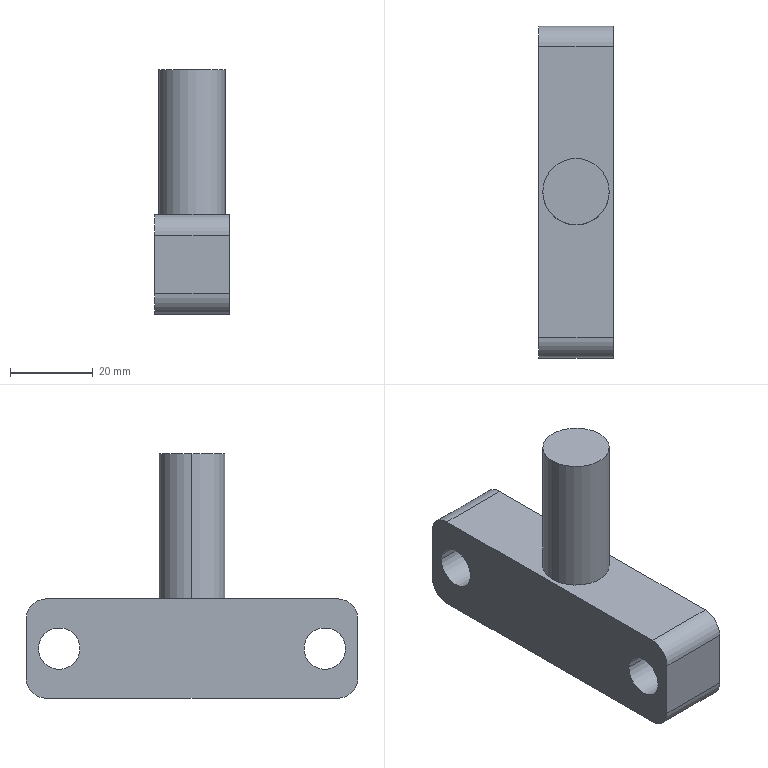Part | SolidWorks | features ICE 2, Extrusion 1, Fillet 1 | 1 solid | 17 faces | box 18 x 80 x 59 mm | volume 38383 mm3 | cylinder 10 | plane 7 | commonest cylinder face diameters 10 x8 16 x2
STEP:
#1=CARTESIAN_POINT('',(9.,37.,-12.));
#2=VERTEX_POINT('',#1);
#3=CARTESIAN_POINT('',(9.,27.,-12.));
#4=VERTEX_POINT('',#3);
#5=CARTESIAN_POINT('',(9.,32.,-12.));
#6=DIRECTION('',(-1.,0.,0.));
#7=DIRECTION('',(0.,-1.,0.));
#8=AXIS2_PLACEMENT_3D('',#5,#6,#7);
#9=CIRCLE('',#8,5.);
#10=EDGE_CURVE('',#2,#4,#9,.T.);
#11=ORIENTED_EDGE('',*,*,#10,.F.);
#12=CARTESIAN_POINT('',(-9.,37.,-12.));
#13=VERTEX_POINT('',#12);
#14=CARTESIAN_POINT('',(9.,37.,-12.));
#15=DIRECTION('',(-1.,0.,0.));
#16=VECTOR('',#15,1000.);
#17=LINE('',#14,#16);
#18=EDGE_CURVE('',#2,#13,#17,.T.);
#19=ORIENTED_EDGE('',*,*,#18,.T.);
#20=CARTESIAN_POINT('',(-9.,27.,-12.));
#21=VERTEX_POINT('',#20);
#22=CARTESIAN_POINT('',(-9.,32.,-12.));
#23=DIRECTION('',(-1.,0.,0.));
#24=DIRECTION('',(0.,-1.,0.));
#25=AXIS2_PLACEMENT_3D('',#22,#23,#24);
#26=CIRCLE('',#25,5.);
#27=EDGE_CURVE('',#13,#21,#26,.T.);
#28=ORIENTED_EDGE('',*,*,#27,.T.);
#29=CARTESIAN_POINT('',(9.,27.,-12.));
#30=DIRECTION('',(-1.,0.,0.));
#31=VECTOR('',#30,1000.);
#32=LINE('',#29,#31);
#33=EDGE_CURVE('',#4,#21,#32,.T.);
#34=ORIENTED_EDGE('',*,*,#33,.F.);
#35=EDGE_LOOP('',(#11,#19,#28,#34));
#36=FACE_OUTER_BOUND('',#35,.T.);
#37=CARTESIAN_POINT('',(9.,32.,-12.));
#38=DIRECTION('',(-1.,0.,0.));
#39=DIRECTION('',(0.,-1.,0.));
#40=AXIS2_PLACEMENT_3D('',#37,#38,#39);
#41=CYLINDRICAL_SURFACE('',#40,5.);
#42=ADVANCED_FACE('',(#36),#41,.F.);
#43=CARTESIAN_POINT('',(9.,-27.,-12.));
#44=VERTEX_POINT('',#43);
#45=CARTESIAN_POINT('',(9.,-37.,-12.));
#46=VERTEX_POINT('',#45);
#47=CARTESIAN_POINT('',(9.,-32.,-12.));
#48=DIRECTION('',(-1.,0.,0.));
#49=DIRECTION('',(0.,-1.,0.));
#50=AXIS2_PLACEMENT_3D('',#47,#48,#49);
#51=CIRCLE('',#50,5.);
#52=EDGE_CURVE('',#44,#46,#51,.T.);
#53=ORIENTED_EDGE('',*,*,#52,.F.);
#54=CARTESIAN_POINT('',(-9.,-27.,-12.));
#55=VERTEX_POINT('',#54);
#56=CARTESIAN_POINT('',(9.,-27.,-12.));
#57=DIRECTION('',(-1.,0.,0.));
#58=VECTOR('',#57,1000.);
#59=LINE('',#56,#58);
#60=EDGE_CURVE('',#44,#55,#59,.T.);
#61=ORIENTED_EDGE('',*,*,#60,.T.);
#62=CARTESIAN_POINT('',(-9.,-37.,-12.));
#63=VERTEX_POINT('',#62);
#64=CARTESIAN_POINT('',(-9.,-32.,-12.));
#65=DIRECTION('',(-1.,0.,0.));
#66=DIRECTION('',(0.,-1.,0.));
#67=AXIS2_PLACEMENT_3D('',#64,#65,#66);
#68=CIRCLE('',#67,5.);
#69=EDGE_CURVE('',#55,#63,#68,.T.);
#70=ORIENTED_EDGE('',*,*,#69,.T.);
#71=CARTESIAN_POINT('',(9.,-37.,-12.));
#72=DIRECTION('',(-1.,0.,0.));
#73=VECTOR('',#72,1000.);
#74=LINE('',#71,#73);
#75=EDGE_CURVE('',#46,#63,#74,.T.);
#76=ORIENTED_EDGE('',*,*,#75,.F.);
#77=EDGE_LOOP('',(#53,#61,#70,#76));
#78=FACE_OUTER_BOUND('',#77,.T.);
#79=CARTESIAN_POINT('',(9.,-32.,-12.));
#80=DIRECTION('',(-1.,0.,0.));
#81=DIRECTION('',(0.,-1.,0.));
#82=AXIS2_PLACEMENT_3D('',#79,#80,#81);
#83=CYLINDRICAL_SURFACE('',#82,5.);
#84=ADVANCED_FACE('',(#78),#83,.F.);
#85=CARTESIAN_POINT('',(8.,0.,35.));
#86=VERTEX_POINT('',#85);
#87=CARTESIAN_POINT('',(-8.,0.,35.));
#88=VERTEX_POINT('',#87);
#89=CARTESIAN_POINT('',(0.,0.,35.));
#90=DIRECTION('',(0.,0.,1.));
#91=DIRECTION('',(1.,0.,0.));
#92=AXIS2_PLACEMENT_3D('',#89,#90,#91);
#93=CIRCLE('',#92,8.);
#94=EDGE_CURVE('',#86,#88,#93,.T.);
#95=ORIENTED_EDGE('',*,*,#94,.F.);
#96=CARTESIAN_POINT('',(8.,0.,0.));
#97=VERTEX_POINT('',#96);
#98=CARTESIAN_POINT('',(8.,0.,35.));
#99=DIRECTION('',(0.,0.,-1.));
#100=VECTOR('',#99,1000.);
#101=LINE('',#98,#100);
#102=EDGE_CURVE('',#86,#97,#101,.T.);
#103=ORIENTED_EDGE('',*,*,#102,.T.);
#104=CARTESIAN_POINT('',(-8.,0.,0.));
#105=VERTEX_POINT('',#104);
#106=CARTESIAN_POINT('',(0.,0.,0.));
#107=DIRECTION('',(0.,0.,1.));
#108=DIRECTION('',(1.,0.,0.));
#109=AXIS2_PLACEMENT_3D('',#106,#107,#108);
#110=CIRCLE('',#109,8.);
#111=EDGE_CURVE('',#97,#105,#110,.T.);
#112=ORIENTED_EDGE('',*,*,#111,.T.);
#113=CARTESIAN_POINT('',(-8.,0.,35.));
#114=DIRECTION('',(0.,0.,-1.));
#115=VECTOR('',#114,1000.);
#116=LINE('',#113,#115);
#117=EDGE_CURVE('',#88,#105,#116,.T.);
#118=ORIENTED_EDGE('',*,*,#117,.F.);
#119=EDGE_LOOP('',(#95,#103,#112,#118));
#120=FACE_OUTER_BOUND('',#119,.T.);
#121=CARTESIAN_POINT('',(0.,0.,35.));
#122=DIRECTION('',(0.,0.,-1.));
#123=DIRECTION('',(-1.,0.,0.));
#124=AXIS2_PLACEMENT_3D('',#121,#122,#123);
#125=CYLINDRICAL_SURFACE('',#124,8.);
#126=ADVANCED_FACE('',(#120),#125,.T.);
#127=ORIENTED_EDGE('',*,*,#102,.F.);
#128=CARTESIAN_POINT('',(0.,0.,35.));
#129=DIRECTION('',(0.,0.,1.));
#130=DIRECTION('',(1.,0.,0.));
#131=AXIS2_PLACEMENT_3D('',#128,#129,#130);
#132=CIRCLE('',#131,8.);
#133=EDGE_CURVE('',#88,#86,#132,.T.);
#134=ORIENTED_EDGE('',*,*,#133,.F.);
#135=ORIENTED_EDGE('',*,*,#117,.T.);
#136=CARTESIAN_POINT('',(0.,0.,0.));
#137=DIRECTION('',(0.,0.,1.));
#138=DIRECTION('',(1.,0.,0.));
#139=AXIS2_PLACEMENT_3D('',#136,#137,#138);
#140=CIRCLE('',#139,8.);
#141=EDGE_CURVE('',#105,#97,#140,.T.);
#142=ORIENTED_EDGE('',*,*,#141,.T.);
#143=EDGE_LOOP('',(#127,#134,#135,#142));
#144=FACE_OUTER_BOUND('',#143,.T.);
#145=CARTESIAN_POINT('',(0.,0.,35.));
#146=DIRECTION('',(0.,0.,-1.));
#147=DIRECTION('',(-1.,0.,0.));
#148=AXIS2_PLACEMENT_3D('',#145,#146,#147);
#149=CYLINDRICAL_SURFACE('',#148,8.);
#150=ADVANCED_FACE('',(#144),#149,.T.);
#151=ORIENTED_EDGE('',*,*,#133,.T.);
#152=ORIENTED_EDGE('',*,*,#94,.T.);
#153=EDGE_LOOP('',(#151,#152));
#154=FACE_OUTER_BOUND('',#153,.T.);
#155=CARTESIAN_POINT('',(0.,0.,35.));
#156=DIRECTION('',(0.,0.,1.));
#157=DIRECTION('',(1.,0.,0.));
#158=AXIS2_PLACEMENT_3D('',#155,#156,#157);
#159=PLANE('',#158);
#160=ADVANCED_FACE('',(#154),#159,.T.);
#161=CARTESIAN_POINT('',(-9.,-35.,0.));
#162=VERTEX_POINT('',#161);
#163=CARTESIAN_POINT('',(-9.,35.,0.));
#164=VERTEX_POINT('',#163);
#165=CARTESIAN_POINT('',(-9.,40.,0.));
#166=DIRECTION('',(0.,1.,0.));
#167=VECTOR('',#166,1000.);
#168=LINE('',#165,#167);
#169=EDGE_CURVE('',#162,#164,#168,.T.);
#170=ORIENTED_EDGE('',*,*,#169,.F.);
#171=CARTESIAN_POINT('',(9.,-35.,0.));
#172=VERTEX_POINT('',#171);
#173=CARTESIAN_POINT('',(9.,-35.,0.));
#174=DIRECTION('',(1.,0.,0.));
#175=VECTOR('',#174,1000.);
#176=LINE('',#173,#175);
#177=EDGE_CURVE('',#162,#172,#176,.T.);
#178=ORIENTED_EDGE('',*,*,#177,.T.);
#179=CARTESIAN_POINT('',(9.,35.,0.));
#180=VERTEX_POINT('',#179);
#181=CARTESIAN_POINT('',(9.,40.,0.));
#182=DIRECTION('',(0.,-1.,0.));
#183=VECTOR('',#182,1000.);
#184=LINE('',#181,#183);
#185=EDGE_CURVE('',#180,#172,#184,.T.);
#186=ORIENTED_EDGE('',*,*,#185,.F.);
#187=CARTESIAN_POINT('',(-9.,35.,0.));
#188=DIRECTION('',(-1.,0.,0.));
#189=VECTOR('',#188,1000.);
#190=LINE('',#187,#189);
#191=EDGE_CURVE('',#180,#164,#190,.T.);
#192=ORIENTED_EDGE('',*,*,#191,.T.);
#193=EDGE_LOOP('',(#170,#178,#186,#192));
#194=FACE_OUTER_BOUND('',#193,.T.);
#195=ORIENTED_EDGE('',*,*,#141,.F.);
#196=ORIENTED_EDGE('',*,*,#111,.F.);
#197=EDGE_LOOP('',(#195,#196));
#198=FACE_BOUND('',#197,.T.);
#199=CARTESIAN_POINT('',(0.,0.,0.));
#200=DIRECTION('',(0.,0.,1.));
#201=DIRECTION('',(1.,0.,0.));
#202=AXIS2_PLACEMENT_3D('',#199,#200,#201);
#203=PLANE('',#202);
#204=ADVANCED_FACE('',(#194,#198),#203,.T.);
#205=CARTESIAN_POINT('',(9.,32.,-12.));
#206=DIRECTION('',(-1.,0.,0.));
#207=DIRECTION('',(0.,-1.,0.));
#208=AXIS2_PLACEMENT_3D('',#205,#206,#207);
#209=CIRCLE('',#208,5.);
#210=EDGE_CURVE('',#4,#2,#209,.T.);
#211=ORIENTED_EDGE('',*,*,#210,.T.);
#212=ORIENTED_EDGE('',*,*,#10,.T.);
#213=EDGE_LOOP('',(#211,#212));
#214=FACE_BOUND('',#213,.T.);
#215=CARTESIAN_POINT('',(9.,-32.,-12.));
#216=DIRECTION('',(-1.,0.,0.));
#217=DIRECTION('',(0.,-1.,0.));
#218=AXIS2_PLACEMENT_3D('',#215,#216,#217);
#219=CIRCLE('',#218,5.);
#220=EDGE_CURVE('',#46,#44,#219,.T.);
#221=ORIENTED_EDGE('',*,*,#220,.T.);
#222=ORIENTED_EDGE('',*,*,#52,.T.);
#223=EDGE_LOOP('',(#221,#222));
#224=FACE_BOUND('',#223,.T.);
#225=ORIENTED_EDGE('',*,*,#185,.T.);
#226=CARTESIAN_POINT('',(9.,-40.,-5.));
#227=VERTEX_POINT('',#226);
#228=CARTESIAN_POINT('',(9.,-35.,-5.));
#229=DIRECTION('',(1.,0.,0.));
#230=DIRECTION('',(0.,-1.,0.));
#231=AXIS2_PLACEMENT_3D('',#228,#229,#230);
#232=CIRCLE('',#231,5.);
#233=EDGE_CURVE('',#172,#227,#232,.T.);
#234=ORIENTED_EDGE('',*,*,#233,.T.);
#235=CARTESIAN_POINT('',(9.,-40.,-19.));
#236=VERTEX_POINT('',#235);
#237=CARTESIAN_POINT('',(9.,-40.,-24.));
#238=DIRECTION('',(0.,0.,1.));
#239=VECTOR('',#238,1000.);
#240=LINE('',#237,#239);
#241=EDGE_CURVE('',#236,#227,#240,.T.);
#242=ORIENTED_EDGE('',*,*,#241,.F.);
#243=CARTESIAN_POINT('',(9.,-35.,-24.));
#244=VERTEX_POINT('',#243);
#245=CARTESIAN_POINT('',(9.,-35.,-19.));
#246=DIRECTION('',(1.,0.,0.));
#247=DIRECTION('',(0.,-1.,0.));
#248=AXIS2_PLACEMENT_3D('',#245,#246,#247);
#249=CIRCLE('',#248,5.);
#250=EDGE_CURVE('',#236,#244,#249,.T.);
#251=ORIENTED_EDGE('',*,*,#250,.T.);
#252=CARTESIAN_POINT('',(9.,35.,-24.));
#253=VERTEX_POINT('',#252);
#254=CARTESIAN_POINT('',(9.,40.,-24.));
#255=DIRECTION('',(0.,-1.,0.));
#256=VECTOR('',#255,1000.);
#257=LINE('',#254,#256);
#258=EDGE_CURVE('',#253,#244,#257,.T.);
#259=ORIENTED_EDGE('',*,*,#258,.F.);
#260=CARTESIAN_POINT('',(9.,40.,-19.));
#261=VERTEX_POINT('',#260);
#262=CARTESIAN_POINT('',(9.,35.,-19.));
#263=DIRECTION('',(1.,0.,0.));
#264=DIRECTION('',(0.,-1.,0.));
#265=AXIS2_PLACEMENT_3D('',#262,#263,#264);
#266=CIRCLE('',#265,5.);
#267=EDGE_CURVE('',#253,#261,#266,.T.);
#268=ORIENTED_EDGE('',*,*,#267,.T.);
#269=CARTESIAN_POINT('',(9.,40.,-5.));
#270=VERTEX_POINT('',#269);
#271=CARTESIAN_POINT('',(9.,40.,-24.));
#272=DIRECTION('',(0.,0.,1.));
#273=VECTOR('',#272,1000.);
#274=LINE('',#271,#273);
#275=EDGE_CURVE('',#261,#270,#274,.T.);
#276=ORIENTED_EDGE('',*,*,#275,.T.);
#277=CARTESIAN_POINT('',(9.,35.,-5.));
#278=DIRECTION('',(1.,0.,0.));
#279=DIRECTION('',(0.,-1.,0.));
#280=AXIS2_PLACEMENT_3D('',#277,#278,#279);
#281=CIRCLE('',#280,5.);
#282=EDGE_CURVE('',#270,#180,#281,.T.);
#283=ORIENTED_EDGE('',*,*,#282,.T.);
#284=EDGE_LOOP('',(#225,#234,#242,#251,#259,#268,#276,#283));
#285=FACE_OUTER_BOUND('',#284,.T.);
#286=CARTESIAN_POINT('',(9.,40.,-24.));
#287=DIRECTION('',(-1.,0.,0.));
#288=DIRECTION('',(0.,-1.,0.));
#289=AXIS2_PLACEMENT_3D('',#286,#287,#288);
#290=PLANE('',#289);
#291=ADVANCED_FACE('',(#214,#224,#285),#290,.F.);
#292=ORIENTED_EDGE('',*,*,#241,.T.);
#293=CARTESIAN_POINT('',(-9.,-40.,-5.));
#294=VERTEX_POINT('',#293);
#295=CARTESIAN_POINT('',(-9.,-40.,-5.));
#296=DIRECTION('',(-1.,0.,0.));
#297=VECTOR('',#296,1000.);
#298=LINE('',#295,#297);
#299=EDGE_CURVE('',#227,#294,#298,.T.);
#300=ORIENTED_EDGE('',*,*,#299,.T.);
#301=CARTESIAN_POINT('',(-9.,-40.,-19.));
#302=VERTEX_POINT('',#301);
#303=CARTESIAN_POINT('',(-9.,-40.,-24.));
#304=DIRECTION('',(0.,0.,1.));
#305=VECTOR('',#304,1000.);
#306=LINE('',#303,#305);
#307=EDGE_CURVE('',#302,#294,#306,.T.);
#308=ORIENTED_EDGE('',*,*,#307,.F.);
#309=CARTESIAN_POINT('',(-9.,-40.,-19.));
#310=DIRECTION('',(1.,0.,0.));
#311=VECTOR('',#310,1000.);
#312=LINE('',#309,#311);
#313=EDGE_CURVE('',#302,#236,#312,.T.);
#314=ORIENTED_EDGE('',*,*,#313,.T.);
#315=EDGE_LOOP('',(#292,#300,#308,#314));
#316=FACE_OUTER_BOUND('',#315,.T.);
#317=CARTESIAN_POINT('',(-9.,-40.,-24.));
#318=DIRECTION('',(0.,1.,0.));
#319=DIRECTION('',(0.,0.,1.));
#320=AXIS2_PLACEMENT_3D('',#317,#318,#319);
#321=PLANE('',#320);
#322=ADVANCED_FACE('',(#316),#321,.F.);
#323=CARTESIAN_POINT('',(-9.,32.,-12.));
#324=DIRECTION('',(-1.,0.,0.));
#325=DIRECTION('',(0.,-1.,0.));
#326=AXIS2_PLACEMENT_3D('',#323,#324,#325);
#327=CIRCLE('',#326,5.);
#328=EDGE_CURVE('',#21,#13,#327,.T.);
#329=ORIENTED_EDGE('',*,*,#328,.F.);
#330=ORIENTED_EDGE('',*,*,#27,.F.);
#331=EDGE_LOOP('',(#329,#330));
#332=FACE_BOUND('',#331,.T.);
#333=CARTESIAN_POINT('',(-9.,-32.,-12.));
#334=DIRECTION('',(-1.,0.,0.));
#335=DIRECTION('',(0.,-1.,0.));
#336=AXIS2_PLACEMENT_3D('',#333,#334,#335);
#337=CIRCLE('',#336,5.);
#338=EDGE_CURVE('',#63,#55,#337,.T.);
#339=ORIENTED_EDGE('',*,*,#338,.F.);
#340=ORIENTED_EDGE('',*,*,#69,.F.);
#341=EDGE_LOOP('',(#339,#340));
#342=FACE_BOUND('',#341,.T.);
#343=ORIENTED_EDGE('',*,*,#307,.T.);
#344=CARTESIAN_POINT('',(-9.,-35.,-5.));
#345=DIRECTION('',(-1.,0.,0.));
#346=DIRECTION('',(0.,1.,0.));
#347=AXIS2_PLACEMENT_3D('',#344,#345,#346);
#348=CIRCLE('',#347,5.);
#349=EDGE_CURVE('',#294,#162,#348,.T.);
#350=ORIENTED_EDGE('',*,*,#349,.T.);
#351=ORIENTED_EDGE('',*,*,#169,.T.);
#352=CARTESIAN_POINT('',(-9.,40.,-5.));
#353=VERTEX_POINT('',#352);
#354=CARTESIAN_POINT('',(-9.,35.,-5.));
#355=DIRECTION('',(-1.,0.,0.));
#356=DIRECTION('',(0.,1.,0.));
#357=AXIS2_PLACEMENT_3D('',#354,#355,#356);
#358=CIRCLE('',#357,5.);
#359=EDGE_CURVE('',#164,#353,#358,.T.);
#360=ORIENTED_EDGE('',*,*,#359,.T.);
#361=CARTESIAN_POINT('',(-9.,40.,-19.));
#362=VERTEX_POINT('',#361);
#363=CARTESIAN_POINT('',(-9.,40.,-24.));
#364=DIRECTION('',(0.,0.,1.));
#365=VECTOR('',#364,1000.);
#366=LINE('',#363,#365);
#367=EDGE_CURVE('',#362,#353,#366,.T.);
#368=ORIENTED_EDGE('',*,*,#367,.F.);
#369=CARTESIAN_POINT('',(-9.,35.,-24.));
#370=VERTEX_POINT('',#369);
#371=CARTESIAN_POINT('',(-9.,35.,-19.));
#372=DIRECTION('',(-1.,0.,0.));
#373=DIRECTION('',(0.,1.,0.));
#374=AXIS2_PLACEMENT_3D('',#371,#372,#373);
#375=CIRCLE('',#374,5.);
#376=EDGE_CURVE('',#362,#370,#375,.T.);
#377=ORIENTED_EDGE('',*,*,#376,.T.);
#378=CARTESIAN_POINT('',(-9.,-35.,-24.));
#379=VERTEX_POINT('',#378);
#380=CARTESIAN_POINT('',(-9.,40.,-24.));
#381=DIRECTION('',(0.,1.,0.));
#382=VECTOR('',#381,1000.);
#383=LINE('',#380,#382);
#384=EDGE_CURVE('',#379,#370,#383,.T.);
#385=ORIENTED_EDGE('',*,*,#384,.F.);
#386=CARTESIAN_POINT('',(-9.,-35.,-19.));
#387=DIRECTION('',(-1.,0.,0.));
#388=DIRECTION('',(0.,1.,0.));
#389=AXIS2_PLACEMENT_3D('',#386,#387,#388);
#390=CIRCLE('',#389,5.);
#391=EDGE_CURVE('',#379,#302,#390,.T.);
#392=ORIENTED_EDGE('',*,*,#391,.T.);
#393=EDGE_LOOP('',(#343,#350,#351,#360,#368,#377,#385,#392));
#394=FACE_OUTER_BOUND('',#393,.T.);
#395=CARTESIAN_POINT('',(-9.,40.,-24.));
#396=DIRECTION('',(1.,0.,0.));
#397=DIRECTION('',(0.,1.,0.));
#398=AXIS2_PLACEMENT_3D('',#395,#396,#397);
#399=PLANE('',#398);
#400=ADVANCED_FACE('',(#332,#342,#394),#399,.F.);
#401=ORIENTED_EDGE('',*,*,#367,.T.);
#402=CARTESIAN_POINT('',(9.,40.,-5.));
#403=DIRECTION('',(1.,0.,0.));
#404=VECTOR('',#403,1000.);
#405=LINE('',#402,#404);
#406=EDGE_CURVE('',#353,#270,#405,.T.);
#407=ORIENTED_EDGE('',*,*,#406,.T.);
#408=ORIENTED_EDGE('',*,*,#275,.F.);
#409=CARTESIAN_POINT('',(-9.,40.,-19.));
#410=DIRECTION('',(-1.,0.,0.));
#411=VECTOR('',#410,1000.);
#412=LINE('',#409,#411);
#413=EDGE_CURVE('',#261,#362,#412,.T.);
#414=ORIENTED_EDGE('',*,*,#413,.T.);
#415=EDGE_LOOP('',(#401,#407,#408,#414));
#416=FACE_OUTER_BOUND('',#415,.T.);
#417=CARTESIAN_POINT('',(-9.,40.,-24.));
#418=DIRECTION('',(0.,-1.,0.));
#419=DIRECTION('',(0.,0.,-1.));
#420=AXIS2_PLACEMENT_3D('',#417,#418,#419);
#421=PLANE('',#420);
#422=ADVANCED_FACE('',(#416),#421,.F.);
#423=ORIENTED_EDGE('',*,*,#258,.T.);
#424=CARTESIAN_POINT('',(0.,-35.,-24.));
#425=DIRECTION('',(-1.,0.,0.));
#426=VECTOR('',#425,1000.);
#427=LINE('',#424,#426);
#428=EDGE_CURVE('',#244,#379,#427,.T.);
#429=ORIENTED_EDGE('',*,*,#428,.T.);
#430=ORIENTED_EDGE('',*,*,#384,.T.);
#431=CARTESIAN_POINT('',(0.,35.,-24.));
#432=DIRECTION('',(1.,0.,0.));
#433=VECTOR('',#432,1000.);
#434=LINE('',#431,#433);
#435=EDGE_CURVE('',#370,#253,#434,.T.);
#436=ORIENTED_EDGE('',*,*,#435,.T.);
#437=EDGE_LOOP('',(#423,#429,#430,#436));
#438=FACE_OUTER_BOUND('',#437,.T.);
#439=CARTESIAN_POINT('',(0.,0.,-24.));
#440=DIRECTION('',(0.,0.,1.));
#441=DIRECTION('',(1.,0.,0.));
#442=AXIS2_PLACEMENT_3D('',#439,#440,#441);
#443=PLANE('',#442);
#444=ADVANCED_FACE('',(#438),#443,.F.);
#445=ORIENTED_EDGE('',*,*,#233,.F.);
#446=ORIENTED_EDGE('',*,*,#177,.F.);
#447=ORIENTED_EDGE('',*,*,#349,.F.);
#448=ORIENTED_EDGE('',*,*,#299,.F.);
#449=EDGE_LOOP('',(#445,#446,#447,#448));
#450=FACE_OUTER_BOUND('',#449,.T.);
#451=CARTESIAN_POINT('',(-9.,-35.,-5.));
#452=DIRECTION('',(1.,0.,0.));
#453=DIRECTION('',(0.,0.,-1.));
#454=AXIS2_PLACEMENT_3D('',#451,#452,#453);
#455=CYLINDRICAL_SURFACE('',#454,5.);
#456=ADVANCED_FACE('',(#450),#455,.T.);
#457=ORIENTED_EDGE('',*,*,#250,.F.);
#458=ORIENTED_EDGE('',*,*,#313,.F.);
#459=ORIENTED_EDGE('',*,*,#391,.F.);
#460=ORIENTED_EDGE('',*,*,#428,.F.);
#461=EDGE_LOOP('',(#457,#458,#459,#460));
#462=FACE_OUTER_BOUND('',#461,.T.);
#463=CARTESIAN_POINT('',(0.,-35.,-19.));
#464=DIRECTION('',(-1.,0.,0.));
#465=DIRECTION('',(0.,0.,1.));
#466=AXIS2_PLACEMENT_3D('',#463,#464,#465);
#467=CYLINDRICAL_SURFACE('',#466,5.);
#468=ADVANCED_FACE('',(#462),#467,.T.);
#469=ORIENTED_EDGE('',*,*,#359,.F.);
#470=ORIENTED_EDGE('',*,*,#191,.F.);
#471=ORIENTED_EDGE('',*,*,#282,.F.);
#472=ORIENTED_EDGE('',*,*,#406,.F.);
#473=EDGE_LOOP('',(#469,#470,#471,#472));
#474=FACE_OUTER_BOUND('',#473,.T.);
#475=CARTESIAN_POINT('',(-9.,35.,-5.));
#476=DIRECTION('',(-1.,0.,0.));
#477=DIRECTION('',(0.,0.,1.));
#478=AXIS2_PLACEMENT_3D('',#475,#476,#477);
#479=CYLINDRICAL_SURFACE('',#478,5.);
#480=ADVANCED_FACE('',(#474),#479,.T.);
#481=ORIENTED_EDGE('',*,*,#376,.F.);
#482=ORIENTED_EDGE('',*,*,#413,.F.);
#483=ORIENTED_EDGE('',*,*,#267,.F.);
#484=ORIENTED_EDGE('',*,*,#435,.F.);
#485=EDGE_LOOP('',(#481,#482,#483,#484));
#486=FACE_OUTER_BOUND('',#485,.T.);
#487=CARTESIAN_POINT('',(0.,35.,-19.));
#488=DIRECTION('',(1.,0.,0.));
#489=DIRECTION('',(0.,0.,-1.));
#490=AXIS2_PLACEMENT_3D('',#487,#488,#489);
#491=CYLINDRICAL_SURFACE('',#490,5.);
#492=ADVANCED_FACE('',(#486),#491,.T.);
#493=ORIENTED_EDGE('',*,*,#60,.F.);
#494=ORIENTED_EDGE('',*,*,#220,.F.);
#495=ORIENTED_EDGE('',*,*,#75,.T.);
#496=ORIENTED_EDGE('',*,*,#338,.T.);
#497=EDGE_LOOP('',(#493,#494,#495,#496));
#498=FACE_OUTER_BOUND('',#497,.T.);
#499=CARTESIAN_POINT('',(9.,-32.,-12.));
#500=DIRECTION('',(-1.,0.,0.));
#501=DIRECTION('',(0.,-1.,0.));
#502=AXIS2_PLACEMENT_3D('',#499,#500,#501);
#503=CYLINDRICAL_SURFACE('',#502,5.);
#504=ADVANCED_FACE('',(#498),#503,.F.);
#505=ORIENTED_EDGE('',*,*,#18,.F.);
#506=ORIENTED_EDGE('',*,*,#210,.F.);
#507=ORIENTED_EDGE('',*,*,#33,.T.);
#508=ORIENTED_EDGE('',*,*,#328,.T.);
#509=EDGE_LOOP('',(#505,#506,#507,#508));
#510=FACE_OUTER_BOUND('',#509,.T.);
#511=CARTESIAN_POINT('',(9.,32.,-12.));
#512=DIRECTION('',(-1.,0.,0.));
#513=DIRECTION('',(0.,-1.,0.));
#514=AXIS2_PLACEMENT_3D('',#511,#512,#513);
#515=CYLINDRICAL_SURFACE('',#514,5.);
#516=ADVANCED_FACE('',(#510),#515,.F.);
#517=CLOSED_SHELL('',(#42,#84,#126,#150,#160,#204,#291,#322,#400,#422,#444,#456,#468,#480,#492,#504,#516));
#518=MANIFOLD_SOLID_BREP('',#517);
#519=CARTESIAN_POINT('',(0.,0.,0.));
#520=DIRECTION('',(0.,0.,1.));
#521=DIRECTION('',(1.,0.,0.));
#522=AXIS2_PLACEMENT_3D('',#519,#520,#521);
#523=(LENGTH_UNIT()NAMED_UNIT(*)SI_UNIT(.MILLI.,.METRE.));
#524=UNCERTAINTY_MEASURE_WITH_UNIT(LENGTH_MEASURE(0.00001),#523,'','');
#525=(NAMED_UNIT(*)PLANE_ANGLE_UNIT()SI_UNIT($,.RADIAN.));
#526=(NAMED_UNIT(*)SI_UNIT($,.STERADIAN.)SOLID_ANGLE_UNIT());
#527=(GEOMETRIC_REPRESENTATION_CONTEXT(3)GLOBAL_UNCERTAINTY_ASSIGNED_CONTEXT((#524))GLOBAL_UNIT_ASSIGNED_CONTEXT((#523,#525,#526))REPRESENTATION_CONTEXT('',''));
#528=ADVANCED_BREP_SHAPE_REPRESENTATION('',(#518,#522),#527);